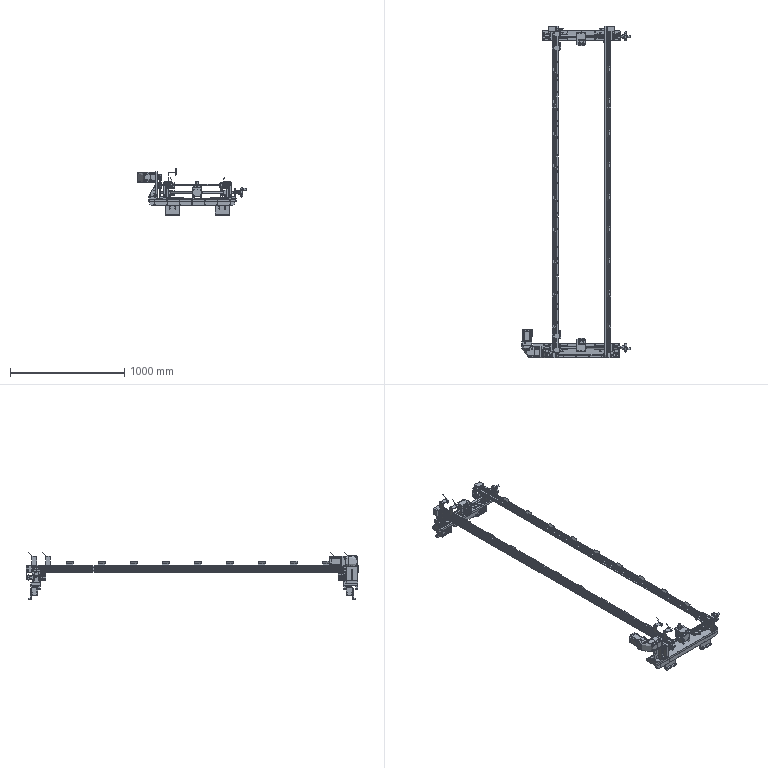Part | SolidWorks | 541 solids | 17042 faces | volume 3235193600058077036305972256511208397885919734211453262778542487408662632075145892487677990725360432235505934277457743697531078312370347809070499934088118999635441221632 mm3 | cylinder 7738 | plane 6041 | cone 1793 | torus 793 | sphere 448 | spline 229 | commonest cylinder face diameters 0.5 x468 6.6 x464 6.55 x460 1.1 x458 1 x370 5 x272